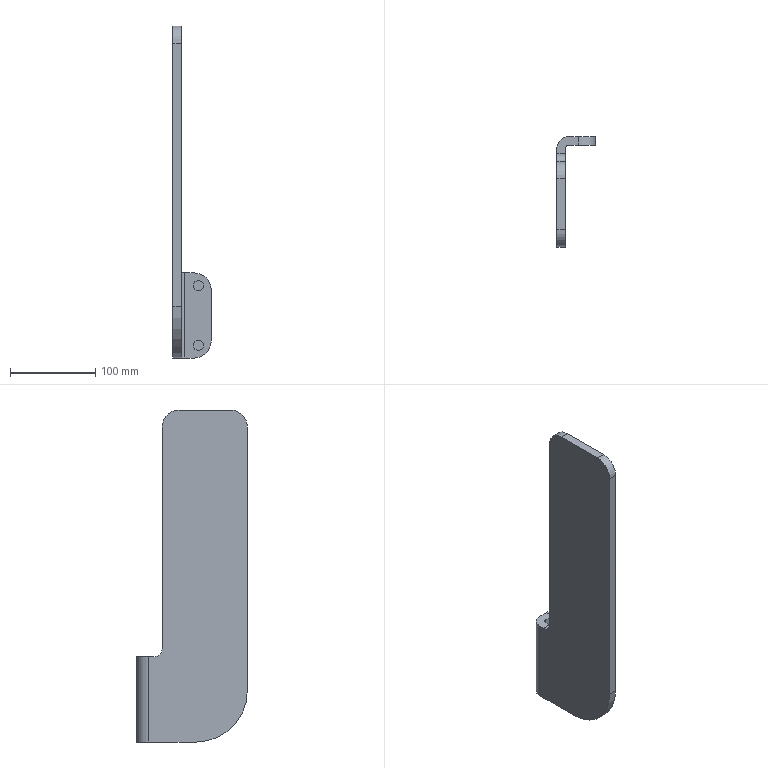Part | SolidWorks | features Fillet 3, ICE 3, LPattern 2, ExtruThin 1 | 1 solid | 30 faces | box 45 x 130 x 390 mm | volume 437695 mm3 | cylinder 16 | plane 14 | commonest cylinder face diameters 11 x4 12 x4 40 x4 8 x1 20 x1 28 x1
STEP:
#1=CARTESIAN_POINT('',(4.,-115.5,375.));
#2=VERTEX_POINT('',#1);
#3=CARTESIAN_POINT('',(4.,-104.5,375.));
#4=VERTEX_POINT('',#3);
#5=CARTESIAN_POINT('',(4.,-110.,375.));
#6=DIRECTION('',(1.,0.,0.));
#7=DIRECTION('',(0.,1.,0.));
#8=AXIS2_PLACEMENT_3D('',#5,#6,#7);
#9=CIRCLE('',#8,5.5);
#10=EDGE_CURVE('',#2,#4,#9,.T.);
#11=ORIENTED_EDGE('',*,*,#10,.F.);
#12=CARTESIAN_POINT('',(10.,-115.5,375.));
#13=VERTEX_POINT('',#12);
#14=CARTESIAN_POINT('',(4.,-115.5,375.));
#15=DIRECTION('',(1.,0.,0.));
#16=VECTOR('',#15,1000.);
#17=LINE('',#14,#16);
#18=EDGE_CURVE('',#2,#13,#17,.T.);
#19=ORIENTED_EDGE('',*,*,#18,.T.);
#20=CARTESIAN_POINT('',(10.,-104.5,375.));
#21=VERTEX_POINT('',#20);
#22=CARTESIAN_POINT('',(10.,-110.,375.));
#23=DIRECTION('',(1.,0.,0.));
#24=DIRECTION('',(0.,1.,0.));
#25=AXIS2_PLACEMENT_3D('',#22,#23,#24);
#26=CIRCLE('',#25,5.5);
#27=EDGE_CURVE('',#13,#21,#26,.T.);
#28=ORIENTED_EDGE('',*,*,#27,.T.);
#29=CARTESIAN_POINT('',(4.,-104.5,375.));
#30=DIRECTION('',(1.,0.,0.));
#31=VECTOR('',#30,1000.);
#32=LINE('',#29,#31);
#33=EDGE_CURVE('',#4,#21,#32,.T.);
#34=ORIENTED_EDGE('',*,*,#33,.F.);
#35=EDGE_LOOP('',(#11,#19,#28,#34));
#36=FACE_OUTER_BOUND('',#35,.T.);
#37=CARTESIAN_POINT('',(4.,-110.,375.));
#38=DIRECTION('',(1.,0.,0.));
#39=DIRECTION('',(0.,1.,0.));
#40=AXIS2_PLACEMENT_3D('',#37,#38,#39);
#41=CYLINDRICAL_SURFACE('',#40,5.5);
#42=ADVANCED_FACE('',(#36),#41,.F.);
#43=CARTESIAN_POINT('',(4.,-55.5,375.));
#44=VERTEX_POINT('',#43);
#45=CARTESIAN_POINT('',(4.,-44.5,375.));
#46=VERTEX_POINT('',#45);
#47=CARTESIAN_POINT('',(4.,-50.,375.));
#48=DIRECTION('',(1.,0.,0.));
#49=DIRECTION('',(0.,1.,0.));
#50=AXIS2_PLACEMENT_3D('',#47,#48,#49);
#51=CIRCLE('',#50,5.5);
#52=EDGE_CURVE('',#44,#46,#51,.T.);
#53=ORIENTED_EDGE('',*,*,#52,.F.);
#54=CARTESIAN_POINT('',(10.,-55.5,375.));
#55=VERTEX_POINT('',#54);
#56=CARTESIAN_POINT('',(4.,-55.5,375.));
#57=DIRECTION('',(1.,0.,0.));
#58=VECTOR('',#57,1000.);
#59=LINE('',#56,#58);
#60=EDGE_CURVE('',#44,#55,#59,.T.);
#61=ORIENTED_EDGE('',*,*,#60,.T.);
#62=CARTESIAN_POINT('',(10.,-44.5,375.));
#63=VERTEX_POINT('',#62);
#64=CARTESIAN_POINT('',(10.,-50.,375.));
#65=DIRECTION('',(1.,0.,0.));
#66=DIRECTION('',(0.,1.,0.));
#67=AXIS2_PLACEMENT_3D('',#64,#65,#66);
#68=CIRCLE('',#67,5.5);
#69=EDGE_CURVE('',#55,#63,#68,.T.);
#70=ORIENTED_EDGE('',*,*,#69,.T.);
#71=CARTESIAN_POINT('',(4.,-44.5,375.));
#72=DIRECTION('',(1.,0.,0.));
#73=VECTOR('',#72,1000.);
#74=LINE('',#71,#73);
#75=EDGE_CURVE('',#46,#63,#74,.T.);
#76=ORIENTED_EDGE('',*,*,#75,.F.);
#77=EDGE_LOOP('',(#53,#61,#70,#76));
#78=FACE_OUTER_BOUND('',#77,.T.);
#79=CARTESIAN_POINT('',(4.,-50.,375.));
#80=DIRECTION('',(1.,0.,0.));
#81=DIRECTION('',(0.,1.,0.));
#82=AXIS2_PLACEMENT_3D('',#79,#80,#81);
#83=CYLINDRICAL_SURFACE('',#82,5.5);
#84=ADVANCED_FACE('',(#78),#83,.F.);
#85=CARTESIAN_POINT('',(30.,-4.,91.));
#86=VERTEX_POINT('',#85);
#87=CARTESIAN_POINT('',(30.,-4.,79.));
#88=VERTEX_POINT('',#87);
#89=CARTESIAN_POINT('',(30.,-4.,85.));
#90=DIRECTION('',(0.,-1.,0.));
#91=DIRECTION('',(0.,0.,-1.));
#92=AXIS2_PLACEMENT_3D('',#89,#90,#91);
#93=CIRCLE('',#92,6.);
#94=EDGE_CURVE('',#86,#88,#93,.T.);
#95=ORIENTED_EDGE('',*,*,#94,.F.);
#96=CARTESIAN_POINT('',(30.,-10.,91.));
#97=VERTEX_POINT('',#96);
#98=CARTESIAN_POINT('',(30.,-4.,91.));
#99=DIRECTION('',(0.,-1.,0.));
#100=VECTOR('',#99,1000.);
#101=LINE('',#98,#100);
#102=EDGE_CURVE('',#86,#97,#101,.T.);
#103=ORIENTED_EDGE('',*,*,#102,.T.);
#104=CARTESIAN_POINT('',(30.,-10.,79.));
#105=VERTEX_POINT('',#104);
#106=CARTESIAN_POINT('',(30.,-10.,85.));
#107=DIRECTION('',(0.,-1.,0.));
#108=DIRECTION('',(0.,0.,-1.));
#109=AXIS2_PLACEMENT_3D('',#106,#107,#108);
#110=CIRCLE('',#109,6.);
#111=EDGE_CURVE('',#97,#105,#110,.T.);
#112=ORIENTED_EDGE('',*,*,#111,.T.);
#113=CARTESIAN_POINT('',(30.,-4.,79.));
#114=DIRECTION('',(0.,-1.,0.));
#115=VECTOR('',#114,1000.);
#116=LINE('',#113,#115);
#117=EDGE_CURVE('',#88,#105,#116,.T.);
#118=ORIENTED_EDGE('',*,*,#117,.F.);
#119=EDGE_LOOP('',(#95,#103,#112,#118));
#120=FACE_OUTER_BOUND('',#119,.T.);
#121=CARTESIAN_POINT('',(30.,-4.,85.));
#122=DIRECTION('',(0.,-1.,0.));
#123=DIRECTION('',(0.,0.,-1.));
#124=AXIS2_PLACEMENT_3D('',#121,#122,#123);
#125=CYLINDRICAL_SURFACE('',#124,6.);
#126=ADVANCED_FACE('',(#120),#125,.F.);
#127=CARTESIAN_POINT('',(30.,-4.,21.));
#128=VERTEX_POINT('',#127);
#129=CARTESIAN_POINT('',(30.,-4.,9.));
#130=VERTEX_POINT('',#129);
#131=CARTESIAN_POINT('',(30.,-4.,15.));
#132=DIRECTION('',(0.,-1.,0.));
#133=DIRECTION('',(0.,0.,-1.));
#134=AXIS2_PLACEMENT_3D('',#131,#132,#133);
#135=CIRCLE('',#134,6.);
#136=EDGE_CURVE('',#128,#130,#135,.T.);
#137=ORIENTED_EDGE('',*,*,#136,.F.);
#138=CARTESIAN_POINT('',(30.,-10.,21.));
#139=VERTEX_POINT('',#138);
#140=CARTESIAN_POINT('',(30.,-4.,21.));
#141=DIRECTION('',(0.,-1.,0.));
#142=VECTOR('',#141,1000.);
#143=LINE('',#140,#142);
#144=EDGE_CURVE('',#128,#139,#143,.T.);
#145=ORIENTED_EDGE('',*,*,#144,.T.);
#146=CARTESIAN_POINT('',(30.,-10.,9.));
#147=VERTEX_POINT('',#146);
#148=CARTESIAN_POINT('',(30.,-10.,15.));
#149=DIRECTION('',(0.,-1.,0.));
#150=DIRECTION('',(0.,0.,-1.));
#151=AXIS2_PLACEMENT_3D('',#148,#149,#150);
#152=CIRCLE('',#151,6.);
#153=EDGE_CURVE('',#139,#147,#152,.T.);
#154=ORIENTED_EDGE('',*,*,#153,.T.);
#155=CARTESIAN_POINT('',(30.,-4.,9.));
#156=DIRECTION('',(0.,-1.,0.));
#157=VECTOR('',#156,1000.);
#158=LINE('',#155,#157);
#159=EDGE_CURVE('',#130,#147,#158,.T.);
#160=ORIENTED_EDGE('',*,*,#159,.F.);
#161=EDGE_LOOP('',(#137,#145,#154,#160));
#162=FACE_OUTER_BOUND('',#161,.T.);
#163=CARTESIAN_POINT('',(30.,-4.,15.));
#164=DIRECTION('',(0.,-1.,0.));
#165=DIRECTION('',(0.,0.,-1.));
#166=AXIS2_PLACEMENT_3D('',#163,#164,#165);
#167=CYLINDRICAL_SURFACE('',#166,6.);
#168=ADVANCED_FACE('',(#162),#167,.F.);
#169=CARTESIAN_POINT('',(0.,-14.,0.));
#170=VERTEX_POINT('',#169);
#171=CARTESIAN_POINT('',(0.,-70.,0.));
#172=VERTEX_POINT('',#171);
#173=CARTESIAN_POINT('',(0.,-14.,0.));
#174=DIRECTION('',(0.,-1.,0.));
#175=VECTOR('',#174,1000.);
#176=LINE('',#173,#175);
#177=EDGE_CURVE('',#170,#172,#176,.T.);
#178=ORIENTED_EDGE('',*,*,#177,.T.);
#179=CARTESIAN_POINT('',(0.,-130.,60.));
#180=VERTEX_POINT('',#179);
#181=CARTESIAN_POINT('',(0.,-70.,60.));
#182=DIRECTION('',(-1.,0.,0.));
#183=DIRECTION('',(0.,1.,0.));
#184=AXIS2_PLACEMENT_3D('',#181,#182,#183);
#185=CIRCLE('',#184,60.);
#186=EDGE_CURVE('',#172,#180,#185,.T.);
#187=ORIENTED_EDGE('',*,*,#186,.T.);
#188=CARTESIAN_POINT('',(0.,-130.,370.));
#189=VERTEX_POINT('',#188);
#190=CARTESIAN_POINT('',(0.,-130.,100.));
#191=DIRECTION('',(0.,0.,-1.));
#192=VECTOR('',#191,1000.);
#193=LINE('',#190,#192);
#194=EDGE_CURVE('',#189,#180,#193,.T.);
#195=ORIENTED_EDGE('',*,*,#194,.F.);
#196=CARTESIAN_POINT('',(0.,-110.,390.));
#197=VERTEX_POINT('',#196);
#198=CARTESIAN_POINT('',(0.,-110.,370.));
#199=DIRECTION('',(-1.,0.,0.));
#200=DIRECTION('',(0.,1.,0.));
#201=AXIS2_PLACEMENT_3D('',#198,#199,#200);
#202=CIRCLE('',#201,20.);
#203=EDGE_CURVE('',#189,#197,#202,.T.);
#204=ORIENTED_EDGE('',*,*,#203,.T.);
#205=CARTESIAN_POINT('',(0.,-50.,390.));
#206=VERTEX_POINT('',#205);
#207=CARTESIAN_POINT('',(0.,-130.,390.));
#208=DIRECTION('',(0.,-1.,0.));
#209=VECTOR('',#208,1000.);
#210=LINE('',#207,#209);
#211=EDGE_CURVE('',#206,#197,#210,.T.);
#212=ORIENTED_EDGE('',*,*,#211,.F.);
#213=CARTESIAN_POINT('',(0.,-30.,370.));
#214=VERTEX_POINT('',#213);
#215=CARTESIAN_POINT('',(0.,-50.,370.));
#216=DIRECTION('',(-1.,0.,0.));
#217=DIRECTION('',(0.,1.,0.));
#218=AXIS2_PLACEMENT_3D('',#215,#216,#217);
#219=CIRCLE('',#218,20.);
#220=EDGE_CURVE('',#206,#214,#219,.T.);
#221=ORIENTED_EDGE('',*,*,#220,.T.);
#222=CARTESIAN_POINT('',(0.,-30.,110.));
#223=VERTEX_POINT('',#222);
#224=CARTESIAN_POINT('',(0.,-30.,390.));
#225=DIRECTION('',(0.,0.,-1.));
#226=VECTOR('',#225,1000.);
#227=LINE('',#224,#226);
#228=EDGE_CURVE('',#214,#223,#227,.T.);
#229=ORIENTED_EDGE('',*,*,#228,.T.);
#230=CARTESIAN_POINT('',(0.,-20.,100.));
#231=VERTEX_POINT('',#230);
#232=CARTESIAN_POINT('',(0.,-20.,110.));
#233=DIRECTION('',(1.,0.,0.));
#234=DIRECTION('',(0.,1.,0.));
#235=AXIS2_PLACEMENT_3D('',#232,#233,#234);
#236=CIRCLE('',#235,10.);
#237=EDGE_CURVE('',#223,#231,#236,.T.);
#238=ORIENTED_EDGE('',*,*,#237,.T.);
#239=CARTESIAN_POINT('',(0.,-14.,100.));
#240=VERTEX_POINT('',#239);
#241=CARTESIAN_POINT('',(0.,-14.,100.));
#242=DIRECTION('',(0.,-1.,0.));
#243=VECTOR('',#242,1000.);
#244=LINE('',#241,#243);
#245=EDGE_CURVE('',#240,#231,#244,.T.);
#246=ORIENTED_EDGE('',*,*,#245,.F.);
#247=CARTESIAN_POINT('',(0.,-14.,100.));
#248=DIRECTION('',(0.,0.,-1.));
#249=VECTOR('',#248,1000.);
#250=LINE('',#247,#249);
#251=EDGE_CURVE('',#240,#170,#250,.T.);
#252=ORIENTED_EDGE('',*,*,#251,.T.);
#253=EDGE_LOOP('',(#178,#187,#195,#204,#212,#221,#229,#238,#246,#252));
#254=FACE_OUTER_BOUND('',#253,.T.);
#255=CARTESIAN_POINT('',(0.,-14.,100.));
#256=DIRECTION('',(1.,0.,0.));
#257=DIRECTION('',(0.,1.,0.));
#258=AXIS2_PLACEMENT_3D('',#255,#256,#257);
#259=PLANE('',#258);
#260=ADVANCED_FACE('',(#254),#259,.F.);
#261=ORIENTED_EDGE('',*,*,#194,.T.);
#262=CARTESIAN_POINT('',(10.,-130.,60.));
#263=VERTEX_POINT('',#262);
#264=CARTESIAN_POINT('',(10.,-130.,60.));
#265=DIRECTION('',(1.,0.,0.));
#266=VECTOR('',#265,1000.);
#267=LINE('',#264,#266);
#268=EDGE_CURVE('',#180,#263,#267,.T.);
#269=ORIENTED_EDGE('',*,*,#268,.T.);
#270=CARTESIAN_POINT('',(10.,-130.,370.));
#271=VERTEX_POINT('',#270);
#272=CARTESIAN_POINT('',(10.,-130.,100.));
#273=DIRECTION('',(0.,0.,-1.));
#274=VECTOR('',#273,1000.);
#275=LINE('',#272,#274);
#276=EDGE_CURVE('',#271,#263,#275,.T.);
#277=ORIENTED_EDGE('',*,*,#276,.F.);
#278=CARTESIAN_POINT('',(0.,-130.,370.));
#279=DIRECTION('',(-1.,0.,0.));
#280=VECTOR('',#279,1000.);
#281=LINE('',#278,#280);
#282=EDGE_CURVE('',#271,#189,#281,.T.);
#283=ORIENTED_EDGE('',*,*,#282,.T.);
#284=EDGE_LOOP('',(#261,#269,#277,#283));
#285=FACE_OUTER_BOUND('',#284,.T.);
#286=CARTESIAN_POINT('',(10.,-130.,100.));
#287=DIRECTION('',(0.,-1.,0.));
#288=DIRECTION('',(0.,0.,-1.));
#289=AXIS2_PLACEMENT_3D('',#286,#287,#288);
#290=PLANE('',#289);
#291=ADVANCED_FACE('',(#285),#290,.T.);
#292=CARTESIAN_POINT('',(10.,-110.,375.));
#293=DIRECTION('',(1.,0.,0.));
#294=DIRECTION('',(0.,1.,0.));
#295=AXIS2_PLACEMENT_3D('',#292,#293,#294);
#296=CIRCLE('',#295,5.5);
#297=EDGE_CURVE('',#21,#13,#296,.T.);
#298=ORIENTED_EDGE('',*,*,#297,.F.);
#299=ORIENTED_EDGE('',*,*,#27,.F.);
#300=EDGE_LOOP('',(#298,#299));
#301=FACE_BOUND('',#300,.T.);
#302=CARTESIAN_POINT('',(10.,-50.,375.));
#303=DIRECTION('',(1.,0.,0.));
#304=DIRECTION('',(0.,1.,0.));
#305=AXIS2_PLACEMENT_3D('',#302,#303,#304);
#306=CIRCLE('',#305,5.5);
#307=EDGE_CURVE('',#63,#55,#306,.T.);
#308=ORIENTED_EDGE('',*,*,#307,.F.);
#309=ORIENTED_EDGE('',*,*,#69,.F.);
#310=EDGE_LOOP('',(#308,#309));
#311=FACE_BOUND('',#310,.T.);
#312=ORIENTED_EDGE('',*,*,#276,.T.);
#313=CARTESIAN_POINT('',(10.,-70.,0.));
#314=VERTEX_POINT('',#313);
#315=CARTESIAN_POINT('',(10.,-70.,60.));
#316=DIRECTION('',(1.,0.,0.));
#317=DIRECTION('',(0.,1.,0.));
#318=AXIS2_PLACEMENT_3D('',#315,#316,#317);
#319=CIRCLE('',#318,60.);
#320=EDGE_CURVE('',#263,#314,#319,.T.);
#321=ORIENTED_EDGE('',*,*,#320,.T.);
#322=CARTESIAN_POINT('',(10.,-14.,0.));
#323=VERTEX_POINT('',#322);
#324=CARTESIAN_POINT('',(10.,-14.,0.));
#325=DIRECTION('',(0.,-1.,0.));
#326=VECTOR('',#325,1000.);
#327=LINE('',#324,#326);
#328=EDGE_CURVE('',#323,#314,#327,.T.);
#329=ORIENTED_EDGE('',*,*,#328,.F.);
#330=CARTESIAN_POINT('',(10.,-14.,100.));
#331=VERTEX_POINT('',#330);
#332=CARTESIAN_POINT('',(10.,-14.,100.));
#333=DIRECTION('',(0.,0.,-1.));
#334=VECTOR('',#333,1000.);
#335=LINE('',#332,#334);
#336=EDGE_CURVE('',#331,#323,#335,.T.);
#337=ORIENTED_EDGE('',*,*,#336,.F.);
#338=CARTESIAN_POINT('',(10.,-20.,100.));
#339=VERTEX_POINT('',#338);
#340=CARTESIAN_POINT('',(10.,-14.,100.));
#341=DIRECTION('',(0.,-1.,0.));
#342=VECTOR('',#341,1000.);
#343=LINE('',#340,#342);
#344=EDGE_CURVE('',#331,#339,#343,.T.);
#345=ORIENTED_EDGE('',*,*,#344,.T.);
#346=CARTESIAN_POINT('',(10.,-30.,110.));
#347=VERTEX_POINT('',#346);
#348=CARTESIAN_POINT('',(10.,-20.,110.));
#349=DIRECTION('',(-1.,0.,0.));
#350=DIRECTION('',(0.,1.,0.));
#351=AXIS2_PLACEMENT_3D('',#348,#349,#350);
#352=CIRCLE('',#351,10.);
#353=EDGE_CURVE('',#339,#347,#352,.T.);
#354=ORIENTED_EDGE('',*,*,#353,.T.);
#355=CARTESIAN_POINT('',(10.,-30.,370.));
#356=VERTEX_POINT('',#355);
#357=CARTESIAN_POINT('',(10.,-30.,390.));
#358=DIRECTION('',(0.,0.,-1.));
#359=VECTOR('',#358,1000.);
#360=LINE('',#357,#359);
#361=EDGE_CURVE('',#356,#347,#360,.T.);
#362=ORIENTED_EDGE('',*,*,#361,.F.);
#363=CARTESIAN_POINT('',(10.,-50.,390.));
#364=VERTEX_POINT('',#363);
#365=CARTESIAN_POINT('',(10.,-50.,370.));
#366=DIRECTION('',(1.,0.,0.));
#367=DIRECTION('',(0.,1.,0.));
#368=AXIS2_PLACEMENT_3D('',#365,#366,#367);
#369=CIRCLE('',#368,20.);
#370=EDGE_CURVE('',#356,#364,#369,.T.);
#371=ORIENTED_EDGE('',*,*,#370,.T.);
#372=CARTESIAN_POINT('',(10.,-110.,390.));
#373=VERTEX_POINT('',#372);
#374=CARTESIAN_POINT('',(10.,-130.,390.));
#375=DIRECTION('',(0.,1.,0.));
#376=VECTOR('',#375,1000.);
#377=LINE('',#374,#376);
#378=EDGE_CURVE('',#373,#364,#377,.T.);
#379=ORIENTED_EDGE('',*,*,#378,.F.);
#380=CARTESIAN_POINT('',(10.,-110.,370.));
#381=DIRECTION('',(1.,0.,0.));
#382=DIRECTION('',(0.,1.,0.));
#383=AXIS2_PLACEMENT_3D('',#380,#381,#382);
#384=CIRCLE('',#383,20.);
#385=EDGE_CURVE('',#373,#271,#384,.T.);
#386=ORIENTED_EDGE('',*,*,#385,.T.);
#387=EDGE_LOOP('',(#312,#321,#329,#337,#345,#354,#362,#371,#379,#386));
#388=FACE_OUTER_BOUND('',#387,.T.);
#389=CARTESIAN_POINT('',(10.,-14.,100.));
#390=DIRECTION('',(1.,0.,0.));
#391=DIRECTION('',(0.,1.,0.));
#392=AXIS2_PLACEMENT_3D('',#389,#390,#391);
#393=PLANE('',#392);
#394=ADVANCED_FACE('',(#301,#311,#388),#393,.T.);
#395=CARTESIAN_POINT('',(14.,-10.,0.));
#396=VERTEX_POINT('',#395);
#397=CARTESIAN_POINT('',(14.,-14.,0.));
#398=DIRECTION('',(0.,0.,1.));
#399=DIRECTION('',(1.,0.,0.));
#400=AXIS2_PLACEMENT_3D('',#397,#398,#399);
#401=CIRCLE('',#400,4.);
#402=EDGE_CURVE('',#396,#323,#401,.T.);
#403=ORIENTED_EDGE('',*,*,#402,.F.);
#404=CARTESIAN_POINT('',(14.,-10.,100.));
#405=VERTEX_POINT('',#404);
#406=CARTESIAN_POINT('',(14.,-10.,100.));
#407=DIRECTION('',(0.,0.,-1.));
#408=VECTOR('',#407,1000.);
#409=LINE('',#406,#408);
#410=EDGE_CURVE('',#405,#396,#409,.T.);
#411=ORIENTED_EDGE('',*,*,#410,.F.);
#412=CARTESIAN_POINT('',(14.,-14.,100.));
#413=DIRECTION('',(0.,0.,1.));
#414=DIRECTION('',(1.,0.,0.));
#415=AXIS2_PLACEMENT_3D('',#412,#413,#414);
#416=CIRCLE('',#415,4.);
#417=EDGE_CURVE('',#405,#331,#416,.T.);
#418=ORIENTED_EDGE('',*,*,#417,.T.);
#419=ORIENTED_EDGE('',*,*,#336,.T.);
#420=EDGE_LOOP('',(#403,#411,#418,#419));
#421=FACE_OUTER_BOUND('',#420,.T.);
#422=CARTESIAN_POINT('',(14.,-14.,100.));
#423=DIRECTION('',(0.,0.,-1.));
#424=DIRECTION('',(-1.,0.,0.));
#425=AXIS2_PLACEMENT_3D('',#422,#423,#424);
#426=CYLINDRICAL_SURFACE('',#425,4.);
#427=ADVANCED_FACE('',(#421),#426,.F.);
#428=CARTESIAN_POINT('',(30.,-10.,85.));
#429=DIRECTION('',(0.,-1.,0.));
#430=DIRECTION('',(0.,0.,-1.));
#431=AXIS2_PLACEMENT_3D('',#428,#429,#430);
#432=CIRCLE('',#431,6.);
#433=EDGE_CURVE('',#105,#97,#432,.T.);
#434=ORIENTED_EDGE('',*,*,#433,.F.);
#435=ORIENTED_EDGE('',*,*,#111,.F.);
#436=EDGE_LOOP('',(#434,#435));
#437=FACE_BOUND('',#436,.T.);
#438=CARTESIAN_POINT('',(30.,-10.,15.));
#439=DIRECTION('',(0.,-1.,0.));
#440=DIRECTION('',(0.,0.,-1.));
#441=AXIS2_PLACEMENT_3D('',#438,#439,#440);
#442=CIRCLE('',#441,6.);
#443=EDGE_CURVE('',#147,#139,#442,.T.);
#444=ORIENTED_EDGE('',*,*,#443,.F.);
#445=ORIENTED_EDGE('',*,*,#153,.F.);
#446=EDGE_LOOP('',(#444,#445));
#447=FACE_BOUND('',#446,.T.);
#448=CARTESIAN_POINT('',(25.,-10.,0.));
#449=VERTEX_POINT('',#448);
#450=CARTESIAN_POINT('',(14.,-10.,0.));
#451=DIRECTION('',(-1.,0.,0.));
#452=VECTOR('',#451,1000.);
#453=LINE('',#450,#452);
#454=EDGE_CURVE('',#449,#396,#453,.T.);
#455=ORIENTED_EDGE('',*,*,#454,.F.);
#456=CARTESIAN_POINT('',(45.,-10.,20.));
#457=VERTEX_POINT('',#456);
#458=CARTESIAN_POINT('',(25.,-10.,20.));
#459=DIRECTION('',(0.,-1.,0.));
#460=DIRECTION('',(0.,0.,-1.));
#461=AXIS2_PLACEMENT_3D('',#458,#459,#460);
#462=CIRCLE('',#461,20.);
#463=EDGE_CURVE('',#449,#457,#462,.T.);
#464=ORIENTED_EDGE('',*,*,#463,.T.);
#465=CARTESIAN_POINT('',(45.,-10.,80.));
#466=VERTEX_POINT('',#465);
#467=CARTESIAN_POINT('',(45.,-10.,100.));
#468=DIRECTION('',(0.,0.,-1.));
#469=VECTOR('',#468,1000.);
#470=LINE('',#467,#469);
#471=EDGE_CURVE('',#466,#457,#470,.T.);
#472=ORIENTED_EDGE('',*,*,#471,.F.);
#473=CARTESIAN_POINT('',(25.,-10.,100.));
#474=VERTEX_POINT('',#473);
#475=CARTESIAN_POINT('',(25.,-10.,80.));
#476=DIRECTION('',(0.,-1.,0.));
#477=DIRECTION('',(0.,0.,-1.));
#478=AXIS2_PLACEMENT_3D('',#475,#476,#477);
#479=CIRCLE('',#478,20.);
#480=EDGE_CURVE('',#466,#474,#479,.T.);
#481=ORIENTED_EDGE('',*,*,#480,.T.);
#482=CARTESIAN_POINT('',(14.,-10.,100.));
#483=DIRECTION('',(-1.,0.,0.));
#484=VECTOR('',#483,1000.);
#485=LINE('',#482,#484);
#486=EDGE_CURVE('',#474,#405,#485,.T.);
#487=ORIENTED_EDGE('',*,*,#486,.T.);
#488=ORIENTED_EDGE('',*,*,#410,.T.);
#489=EDGE_LOOP('',(#455,#464,#472,#481,#487,#488));
#490=FACE_OUTER_BOUND('',#489,.T.);
#491=CARTESIAN_POINT('',(14.,-10.,100.));
#492=DIRECTION('',(0.,-1.,0.));
#493=DIRECTION('',(0.,0.,-1.));
#494=AXIS2_PLACEMENT_3D('',#491,#492,#493);
#495=PLANE('',#494);
#496=ADVANCED_FACE('',(#437,#447,#490),#495,.T.);
#497=ORIENTED_EDGE('',*,*,#471,.T.);
#498=CARTESIAN_POINT('',(45.,0.,20.));
#499=VERTEX_POINT('',#498);
#500=CARTESIAN_POINT('',(45.,0.,20.));
#501=DIRECTION('',(0.,1.,0.));
#502=VECTOR('',#501,1000.);
#503=LINE('',#500,#502);
#504=EDGE_CURVE('',#457,#499,#503,.T.);
#505=ORIENTED_EDGE('',*,*,#504,.T.);
#506=CARTESIAN_POINT('',(45.,0.,80.));
#507=VERTEX_POINT('',#506);
#508=CARTESIAN_POINT('',(45.,0.,100.));
#509=DIRECTION('',(0.,0.,-1.));
#510=VECTOR('',#509,1000.);
#511=LINE('',#508,#510);
#512=EDGE_CURVE('',#507,#499,#511,.T.);
#513=ORIENTED_EDGE('',*,*,#512,.F.);
#514=CARTESIAN_POINT('',(45.,0.,80.));
#515=DIRECTION('',(0.,-1.,0.));
#516=VECTOR('',#515,1000.);
#517=LINE('',#514,#516);
#518=EDGE_CURVE('',#507,#466,#517,.T.);
#519=ORIENTED_EDGE('',*,*,#518,.T.);
#520=EDGE_LOOP('',(#497,#505,#513,#519));
#521=FACE_OUTER_BOUND('',#520,.T.);
#522=CARTESIAN_POINT('',(45.,0.,100.));
#523=DIRECTION('',(1.,0.,0.));
#524=DIRECTION('',(0.,0.,-1.));
#525=AXIS2_PLACEMENT_3D('',#522,#523,#524);
#526=PLANE('',#525);
#527=ADVANCED_FACE('',(#521),#526,.T.);
#528=ORIENTED_EDGE('',*,*,#512,.T.);
#529=CARTESIAN_POINT('',(25.,0.,0.));
#530=VERTEX_POINT('',#529);
#531=CARTESIAN_POINT('',(25.,0.,20.));
#532=DIRECTION('',(0.,1.,0.));
#533=DIRECTION('',(0.,0.,-1.));
#534=AXIS2_PLACEMENT_3D('',#531,#532,#533);
#535=CIRCLE('',#534,20.);
#536=EDGE_CURVE('',#499,#530,#535,.T.);
#537=ORIENTED_EDGE('',*,*,#536,.T.);
#538=CARTESIAN_POINT('',(14.,0.,0.));
#539=VERTEX_POINT('',#538);
#540=CARTESIAN_POINT('',(14.,0.,0.));
#541=DIRECTION('',(-1.,0.,0.));
#542=VECTOR('',#541,1000.);
#543=LINE('',#540,#542);
#544=EDGE_CURVE('',#530,#539,#543,.T.);
#545=ORIENTED_EDGE('',*,*,#544,.T.);
#546=CARTESIAN_POINT('',(14.,0.,100.));
#547=VERTEX_POINT('',#546);
#548=CARTESIAN_POINT('',(14.,0.,100.));
#549=DIRECTION('',(0.,0.,-1.));
#550=VECTOR('',#549,1000.);
#551=LINE('',#548,#550);
#552=EDGE_CURVE('',#547,#539,#551,.T.);
#553=ORIENTED_EDGE('',*,*,#552,.F.);
#554=CARTESIAN_POINT('',(25.,0.,100.));
#555=VERTEX_POINT('',#554);
#556=CARTESIAN_POINT('',(14.,0.,100.));
#557=DIRECTION('',(-1.,0.,0.));
#558=VECTOR('',#557,1000.);
#559=LINE('',#556,#558);
#560=EDGE_CURVE('',#555,#547,#559,.T.);
#561=ORIENTED_EDGE('',*,*,#560,.F.);
#562=CARTESIAN_POINT('',(25.,0.,80.));
#563=DIRECTION('',(0.,1.,0.));
#564=DIRECTION('',(0.,0.,-1.));
#565=AXIS2_PLACEMENT_3D('',#562,#563,#564);
#566=CIRCLE('',#565,20.);
#567=EDGE_CURVE('',#555,#507,#566,.T.);
#568=ORIENTED_EDGE('',*,*,#567,.T.);
#569=EDGE_LOOP('',(#528,#537,#545,#553,#561,#568));
#570=FACE_OUTER_BOUND('',#569,.T.);
#571=CARTESIAN_POINT('',(14.,0.,100.));
#572=DIRECTION('',(0.,-1.,0.));
#573=DIRECTION('',(0.,0.,-1.));
#574=AXIS2_PLACEMENT_3D('',#571,#572,#573);
#575=PLANE('',#574);
#576=ADVANCED_FACE('',(#570),#575,.F.);
#577=CARTESIAN_POINT('',(14.,-14.,0.));
#578=DIRECTION('',(0.,0.,1.));
#579=DIRECTION('',(1.,0.,0.));
#580=AXIS2_PLACEMENT_3D('',#577,#578,#579);
#581=CIRCLE('',#580,14.);
#582=EDGE_CURVE('',#539,#170,#581,.T.);
#583=ORIENTED_EDGE('',*,*,#582,.T.);
#584=ORIENTED_EDGE('',*,*,#251,.F.);
#585=CARTESIAN_POINT('',(14.,-14.,100.));
#586=DIRECTION('',(0.,0.,1.));
#587=DIRECTION('',(1.,0.,0.));
#588=AXIS2_PLACEMENT_3D('',#585,#586,#587);
#589=CIRCLE('',#588,14.);
#590=EDGE_CURVE('',#547,#240,#589,.T.);
#591=ORIENTED_EDGE('',*,*,#590,.F.);
#592=ORIENTED_EDGE('',*,*,#552,.T.);
#593=EDGE_LOOP('',(#583,#584,#591,#592));
#594=FACE_OUTER_BOUND('',#593,.T.);
#595=CARTESIAN_POINT('',(14.,-14.,100.));
#596=DIRECTION('',(0.,0.,-1.));
#597=DIRECTION('',(-1.,0.,0.));
#598=AXIS2_PLACEMENT_3D('',#595,#596,#597);
#599=CYLINDRICAL_SURFACE('',#598,14.);
#600=ADVANCED_FACE('',(#594),#599,.T.);
#601=ORIENTED_EDGE('',*,*,#486,.F.);
#602=CARTESIAN_POINT('',(25.,-14.,100.));
#603=DIRECTION('',(0.,1.,0.));
#604=VECTOR('',#603,1000.);
#605=LINE('',#602,#604);
#606=EDGE_CURVE('',#474,#555,#605,.T.);
#607=ORIENTED_EDGE('',*,*,#606,.T.);
#608=ORIENTED_EDGE('',*,*,#560,.T.);
#609=ORIENTED_EDGE('',*,*,#590,.T.);
#610=ORIENTED_EDGE('',*,*,#245,.T.);
#611=CARTESIAN_POINT('',(14.,-20.,100.));
#612=DIRECTION('',(1.,0.,0.));
#613=VECTOR('',#612,1000.);
#614=LINE('',#611,#613);
#615=EDGE_CURVE('',#231,#339,#614,.T.);
#616=ORIENTED_EDGE('',*,*,#615,.T.);
#617=ORIENTED_EDGE('',*,*,#344,.F.);
#618=ORIENTED_EDGE('',*,*,#417,.F.);
#619=EDGE_LOOP('',(#601,#607,#608,#609,#610,#616,#617,#618));
#620=FACE_OUTER_BOUND('',#619,.T.);
#621=CARTESIAN_POINT('',(14.,-14.,100.));
#622=DIRECTION('',(0.,0.,1.));
#623=DIRECTION('',(1.,0.,0.));
#624=AXIS2_PLACEMENT_3D('',#621,#622,#623);
#625=PLANE('',#624);
#626=ADVANCED_FACE('',(#620),#625,.T.);
#627=ORIENTED_EDGE('',*,*,#328,.T.);
#628=CARTESIAN_POINT('',(0.,-70.,0.));
#629=DIRECTION('',(-1.,0.,0.));
#630=VECTOR('',#629,1000.);
#631=LINE('',#628,#630);
#632=EDGE_CURVE('',#314,#172,#631,.T.);
#633=ORIENTED_EDGE('',*,*,#632,.T.);
#634=ORIENTED_EDGE('',*,*,#177,.F.);
#635=ORIENTED_EDGE('',*,*,#582,.F.);
#636=ORIENTED_EDGE('',*,*,#544,.F.);
#637=CARTESIAN_POINT('',(25.,-10.,0.));
#638=DIRECTION('',(0.,-1.,0.));
#639=VECTOR('',#638,1000.);
#640=LINE('',#637,#639);
#641=EDGE_CURVE('',#530,#449,#640,.T.);
#642=ORIENTED_EDGE('',*,*,#641,.T.);
#643=ORIENTED_EDGE('',*,*,#454,.T.);
#644=ORIENTED_EDGE('',*,*,#402,.T.);
#645=EDGE_LOOP('',(#627,#633,#634,#635,#636,#642,#643,#644));
#646=FACE_OUTER_BOUND('',#645,.T.);
#647=CARTESIAN_POINT('',(14.,-14.,0.));
#648=DIRECTION('',(0.,0.,1.));
#649=DIRECTION('',(1.,0.,0.));
#650=AXIS2_PLACEMENT_3D('',#647,#648,#649);
#651=PLANE('',#650);
#652=ADVANCED_FACE('',(#646),#651,.F.);
#653=ORIENTED_EDGE('',*,*,#228,.F.);
#654=CARTESIAN_POINT('',(0.,-30.,370.));
#655=DIRECTION('',(1.,0.,0.));
#656=VECTOR('',#655,1000.);
#657=LINE('',#654,#656);
#658=EDGE_CURVE('',#214,#356,#657,.T.);
#659=ORIENTED_EDGE('',*,*,#658,.T.);
#660=ORIENTED_EDGE('',*,*,#361,.T.);
#661=CARTESIAN_POINT('',(0.,-30.,110.));
#662=DIRECTION('',(-1.,0.,0.));
#663=VECTOR('',#662,1000.);
#664=LINE('',#661,#663);
#665=EDGE_CURVE('',#347,#223,#664,.T.);
#666=ORIENTED_EDGE('',*,*,#665,.T.);
#667=EDGE_LOOP('',(#653,#659,#660,#666));
#668=FACE_OUTER_BOUND('',#667,.T.);
#669=CARTESIAN_POINT('',(0.,-30.,390.));
#670=DIRECTION('',(0.,-1.,0.));
#671=DIRECTION('',(0.,0.,-1.));
#672=AXIS2_PLACEMENT_3D('',#669,#670,#671);
#673=PLANE('',#672);
#674=ADVANCED_FACE('',(#668),#673,.F.);
#675=ORIENTED_EDGE('',*,*,#378,.T.);
#676=CARTESIAN_POINT('',(0.,-50.,390.));
#677=DIRECTION('',(-1.,0.,0.));
#678=VECTOR('',#677,1000.);
#679=LINE('',#676,#678);
#680=EDGE_CURVE('',#364,#206,#679,.T.);
#681=ORIENTED_EDGE('',*,*,#680,.T.);
#682=ORIENTED_EDGE('',*,*,#211,.T.);
#683=CARTESIAN_POINT('',(10.,-110.,390.));
#684=DIRECTION('',(1.,0.,0.));
#685=VECTOR('',#684,1000.);
#686=LINE('',#683,#685);
#687=EDGE_CURVE('',#197,#373,#686,.T.);
#688=ORIENTED_EDGE('',*,*,#687,.T.);
#689=EDGE_LOOP('',(#675,#681,#682,#688));
#690=FACE_OUTER_BOUND('',#689,.T.);
#691=CARTESIAN_POINT('',(0.,0.,390.));
#692=DIRECTION('',(0.,0.,-1.));
#693=DIRECTION('',(-1.,0.,0.));
#694=AXIS2_PLACEMENT_3D('',#691,#692,#693);
#695=PLANE('',#694);
#696=ADVANCED_FACE('',(#690),#695,.F.);
#697=ORIENTED_EDGE('',*,*,#353,.F.);
#698=ORIENTED_EDGE('',*,*,#615,.F.);
#699=ORIENTED_EDGE('',*,*,#237,.F.);
#700=ORIENTED_EDGE('',*,*,#665,.F.);
#701=EDGE_LOOP('',(#697,#698,#699,#700));
#702=FACE_OUTER_BOUND('',#701,.T.);
#703=CARTESIAN_POINT('',(0.,-20.,110.));
#704=DIRECTION('',(-1.,0.,0.));
#705=DIRECTION('',(0.,0.,1.));
#706=AXIS2_PLACEMENT_3D('',#703,#704,#705);
#707=CYLINDRICAL_SURFACE('',#706,10.);
#708=ADVANCED_FACE('',(#702),#707,.F.);
#709=ORIENTED_EDGE('',*,*,#370,.F.);
#710=ORIENTED_EDGE('',*,*,#658,.F.);
#711=ORIENTED_EDGE('',*,*,#220,.F.);
#712=ORIENTED_EDGE('',*,*,#680,.F.);
#713=EDGE_LOOP('',(#709,#710,#711,#712));
#714=FACE_OUTER_BOUND('',#713,.T.);
#715=CARTESIAN_POINT('',(0.,-50.,370.));
#716=DIRECTION('',(-1.,0.,0.));
#717=DIRECTION('',(0.,0.,1.));
#718=AXIS2_PLACEMENT_3D('',#715,#716,#717);
#719=CYLINDRICAL_SURFACE('',#718,20.);
#720=ADVANCED_FACE('',(#714),#719,.T.);
#721=ORIENTED_EDGE('',*,*,#203,.F.);
#722=ORIENTED_EDGE('',*,*,#282,.F.);
#723=ORIENTED_EDGE('',*,*,#385,.F.);
#724=ORIENTED_EDGE('',*,*,#687,.F.);
#725=EDGE_LOOP('',(#721,#722,#723,#724));
#726=FACE_OUTER_BOUND('',#725,.T.);
#727=CARTESIAN_POINT('',(0.,-110.,370.));
#728=DIRECTION('',(-1.,0.,0.));
#729=DIRECTION('',(0.,0.,1.));
#730=AXIS2_PLACEMENT_3D('',#727,#728,#729);
#731=CYLINDRICAL_SURFACE('',#730,20.);
#732=ADVANCED_FACE('',(#726),#731,.T.);
#733=ORIENTED_EDGE('',*,*,#536,.F.);
#734=ORIENTED_EDGE('',*,*,#504,.F.);
#735=ORIENTED_EDGE('',*,*,#463,.F.);
#736=ORIENTED_EDGE('',*,*,#641,.F.);
#737=EDGE_LOOP('',(#733,#734,#735,#736));
#738=FACE_OUTER_BOUND('',#737,.T.);
#739=CARTESIAN_POINT('',(25.,-14.,20.));
#740=DIRECTION('',(0.,1.,0.));
#741=DIRECTION('',(0.,0.,1.));
#742=AXIS2_PLACEMENT_3D('',#739,#740,#741);
#743=CYLINDRICAL_SURFACE('',#742,20.);
#744=ADVANCED_FACE('',(#738),#743,.T.);
#745=ORIENTED_EDGE('',*,*,#567,.F.);
#746=ORIENTED_EDGE('',*,*,#606,.F.);
#747=ORIENTED_EDGE('',*,*,#480,.F.);
#748=ORIENTED_EDGE('',*,*,#518,.F.);
#749=EDGE_LOOP('',(#745,#746,#747,#748));
#750=FACE_OUTER_BOUND('',#749,.T.);
#751=CARTESIAN_POINT('',(25.,0.,80.));
#752=DIRECTION('',(0.,-1.,0.));
#753=DIRECTION('',(0.,0.,-1.));
#754=AXIS2_PLACEMENT_3D('',#751,#752,#753);
#755=CYLINDRICAL_SURFACE('',#754,20.);
#756=ADVANCED_FACE('',(#750),#755,.T.);
#757=ORIENTED_EDGE('',*,*,#320,.F.);
#758=ORIENTED_EDGE('',*,*,#268,.F.);
#759=ORIENTED_EDGE('',*,*,#186,.F.);
#760=ORIENTED_EDGE('',*,*,#632,.F.);
#761=EDGE_LOOP('',(#757,#758,#759,#760));
#762=FACE_OUTER_BOUND('',#761,.T.);
#763=CARTESIAN_POINT('',(14.,-70.,60.));
#764=DIRECTION('',(1.,0.,0.));
#765=DIRECTION('',(0.,0.,-1.));
#766=AXIS2_PLACEMENT_3D('',#763,#764,#765);
#767=CYLINDRICAL_SURFACE('',#766,60.);
#768=ADVANCED_FACE('',(#762),#767,.T.);
#769=ORIENTED_EDGE('',*,*,#144,.F.);
#770=CARTESIAN_POINT('',(30.,-4.,15.));
#771=DIRECTION('',(0.,-1.,0.));
#772=DIRECTION('',(0.,0.,-1.));
#773=AXIS2_PLACEMENT_3D('',#770,#771,#772);
#774=CIRCLE('',#773,6.);
#775=EDGE_CURVE('',#130,#128,#774,.T.);
#776=ORIENTED_EDGE('',*,*,#775,.F.);
#777=ORIENTED_EDGE('',*,*,#159,.T.);
#778=ORIENTED_EDGE('',*,*,#443,.T.);
#779=EDGE_LOOP('',(#769,#776,#777,#778));
#780=FACE_OUTER_BOUND('',#779,.T.);
#781=CARTESIAN_POINT('',(30.,-4.,15.));
#782=DIRECTION('',(0.,-1.,0.));
#783=DIRECTION('',(0.,0.,-1.));
#784=AXIS2_PLACEMENT_3D('',#781,#782,#783);
#785=CYLINDRICAL_SURFACE('',#784,6.);
#786=ADVANCED_FACE('',(#780),#785,.F.);
#787=ORIENTED_EDGE('',*,*,#775,.T.);
#788=ORIENTED_EDGE('',*,*,#136,.T.);
#789=EDGE_LOOP('',(#787,#788));
#790=FACE_OUTER_BOUND('',#789,.T.);
#791=CARTESIAN_POINT('',(30.,-4.,15.));
#792=DIRECTION('',(0.,-1.,0.));
#793=DIRECTION('',(0.,0.,-1.));
#794=AXIS2_PLACEMENT_3D('',#791,#792,#793);
#795=PLANE('',#794);
#796=ADVANCED_FACE('',(#790),#795,.T.);
#797=ORIENTED_EDGE('',*,*,#102,.F.);
#798=CARTESIAN_POINT('',(30.,-4.,85.));
#799=DIRECTION('',(0.,-1.,0.));
#800=DIRECTION('',(0.,0.,-1.));
#801=AXIS2_PLACEMENT_3D('',#798,#799,#800);
#802=CIRCLE('',#801,6.);
#803=EDGE_CURVE('',#88,#86,#802,.T.);
#804=ORIENTED_EDGE('',*,*,#803,.F.);
#805=ORIENTED_EDGE('',*,*,#117,.T.);
#806=ORIENTED_EDGE('',*,*,#433,.T.);
#807=EDGE_LOOP('',(#797,#804,#805,#806));
#808=FACE_OUTER_BOUND('',#807,.T.);
#809=CARTESIAN_POINT('',(30.,-4.,85.));
#810=DIRECTION('',(0.,-1.,0.));
#811=DIRECTION('',(0.,0.,-1.));
#812=AXIS2_PLACEMENT_3D('',#809,#810,#811);
#813=CYLINDRICAL_SURFACE('',#812,6.);
#814=ADVANCED_FACE('',(#808),#813,.F.);
#815=ORIENTED_EDGE('',*,*,#803,.T.);
#816=ORIENTED_EDGE('',*,*,#94,.T.);
#817=EDGE_LOOP('',(#815,#816));
#818=FACE_OUTER_BOUND('',#817,.T.);
#819=CARTESIAN_POINT('',(30.,-4.,85.));
#820=DIRECTION('',(0.,-1.,0.));
#821=DIRECTION('',(0.,0.,-1.));
#822=AXIS2_PLACEMENT_3D('',#819,#820,#821);
#823=PLANE('',#822);
#824=ADVANCED_FACE('',(#818),#823,.T.);
#825=ORIENTED_EDGE('',*,*,#60,.F.);
#826=CARTESIAN_POINT('',(4.,-50.,375.));
#827=DIRECTION('',(1.,0.,0.));
#828=DIRECTION('',(0.,1.,0.));
#829=AXIS2_PLACEMENT_3D('',#826,#827,#828);
#830=CIRCLE('',#829,5.5);
#831=EDGE_CURVE('',#46,#44,#830,.T.);
#832=ORIENTED_EDGE('',*,*,#831,.F.);
#833=ORIENTED_EDGE('',*,*,#75,.T.);
#834=ORIENTED_EDGE('',*,*,#307,.T.);
#835=EDGE_LOOP('',(#825,#832,#833,#834));
#836=FACE_OUTER_BOUND('',#835,.T.);
#837=CARTESIAN_POINT('',(4.,-50.,375.));
#838=DIRECTION('',(1.,0.,0.));
#839=DIRECTION('',(0.,1.,0.));
#840=AXIS2_PLACEMENT_3D('',#837,#838,#839);
#841=CYLINDRICAL_SURFACE('',#840,5.5);
#842=ADVANCED_FACE('',(#836),#841,.F.);
#843=ORIENTED_EDGE('',*,*,#831,.T.);
#844=ORIENTED_EDGE('',*,*,#52,.T.);
#845=EDGE_LOOP('',(#843,#844));
#846=FACE_OUTER_BOUND('',#845,.T.);
#847=CARTESIAN_POINT('',(4.,-50.,375.));
#848=DIRECTION('',(1.,0.,0.));
#849=DIRECTION('',(0.,1.,0.));
#850=AXIS2_PLACEMENT_3D('',#847,#848,#849);
#851=PLANE('',#850);
#852=ADVANCED_FACE('',(#846),#851,.T.);
#853=ORIENTED_EDGE('',*,*,#18,.F.);
#854=CARTESIAN_POINT('',(4.,-110.,375.));
#855=DIRECTION('',(1.,0.,0.));
#856=DIRECTION('',(0.,1.,0.));
#857=AXIS2_PLACEMENT_3D('',#854,#855,#856);
#858=CIRCLE('',#857,5.5);
#859=EDGE_CURVE('',#4,#2,#858,.T.);
#860=ORIENTED_EDGE('',*,*,#859,.F.);
#861=ORIENTED_EDGE('',*,*,#33,.T.);
#862=ORIENTED_EDGE('',*,*,#297,.T.);
#863=EDGE_LOOP('',(#853,#860,#861,#862));
#864=FACE_OUTER_BOUND('',#863,.T.);
#865=CARTESIAN_POINT('',(4.,-110.,375.));
#866=DIRECTION('',(1.,0.,0.));
#867=DIRECTION('',(0.,1.,0.));
#868=AXIS2_PLACEMENT_3D('',#865,#866,#867);
#869=CYLINDRICAL_SURFACE('',#868,5.5);
#870=ADVANCED_FACE('',(#864),#869,.F.);
#871=ORIENTED_EDGE('',*,*,#859,.T.);
#872=ORIENTED_EDGE('',*,*,#10,.T.);
#873=EDGE_LOOP('',(#871,#872));
#874=FACE_OUTER_BOUND('',#873,.T.);
#875=CARTESIAN_POINT('',(4.,-110.,375.));
#876=DIRECTION('',(1.,0.,0.));
#877=DIRECTION('',(0.,1.,0.));
#878=AXIS2_PLACEMENT_3D('',#875,#876,#877);
#879=PLANE('',#878);
#880=ADVANCED_FACE('',(#874),#879,.T.);
#881=CLOSED_SHELL('',(#42,#84,#126,#168,#260,#291,#394,#427,#496,#527,#576,#600,#626,#652,#674,#696,#708,#720,#732,#744,#756,#768,#786,#796,#814,#824,#842,#852,#870,#880));
#882=MANIFOLD_SOLID_BREP('',#881);
#883=CARTESIAN_POINT('',(0.,0.,0.));
#884=DIRECTION('',(0.,0.,1.));
#885=DIRECTION('',(1.,0.,0.));
#886=AXIS2_PLACEMENT_3D('',#883,#884,#885);
#887=(LENGTH_UNIT()NAMED_UNIT(*)SI_UNIT(.MILLI.,.METRE.));
#888=UNCERTAINTY_MEASURE_WITH_UNIT(LENGTH_MEASURE(0.00001),#887,'','');
#889=(NAMED_UNIT(*)PLANE_ANGLE_UNIT()SI_UNIT($,.RADIAN.));
#890=(NAMED_UNIT(*)SI_UNIT($,.STERADIAN.)SOLID_ANGLE_UNIT());
#891=(GEOMETRIC_REPRESENTATION_CONTEXT(3)GLOBAL_UNCERTAINTY_ASSIGNED_CONTEXT((#888))GLOBAL_UNIT_ASSIGNED_CONTEXT((#887,#889,#890))REPRESENTATION_CONTEXT('',''));
#892=ADVANCED_BREP_SHAPE_REPRESENTATION('',(#882,#886),#891);